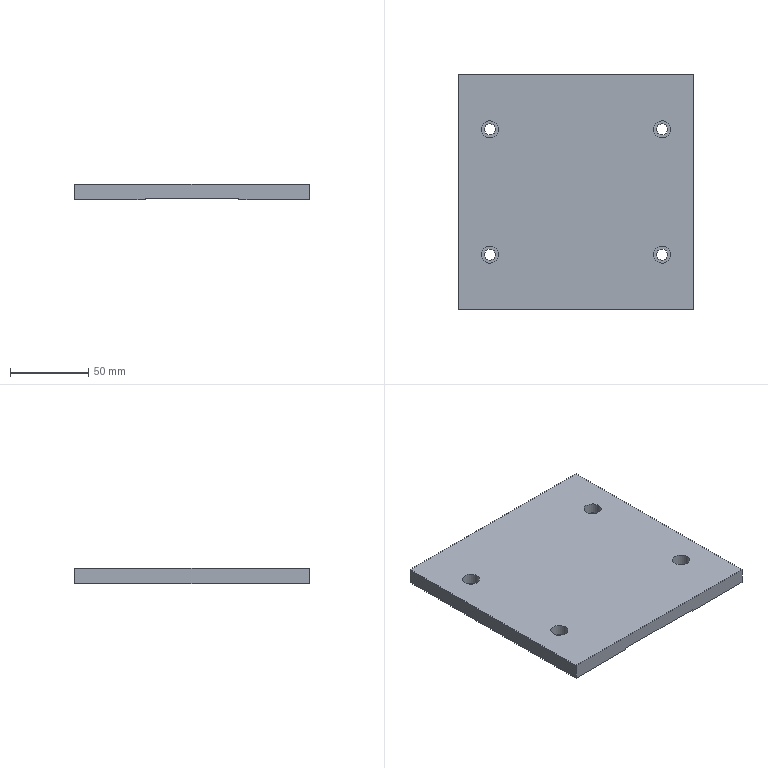Part | NX | features DATUM_CSYS 4, EXTRACT_BODY 3, EXTRUDE 3, SKETCH 3, Container 2, Geometry Instance 2, SUBTRACT 1 | 1 solid | 22 faces | box 150 x 150 x 10 mm | volume 212877 mm3 | plane 14 | cylinder 8 | commonest cylinder face diameters 7 x4 11 x4
STEP:
#1=CARTESIAN_POINT('',(0.,0.,10.));
#2=VERTEX_POINT('',#1);
#3=CARTESIAN_POINT('',(0.,0.,0.));
#4=VERTEX_POINT('',#3);
#5=CARTESIAN_POINT('',(0.,0.,10.));
#6=DIRECTION('',(0.,0.,-1.));
#7=VECTOR('',#6,1000.);
#8=LINE('',#5,#7);
#9=EDGE_CURVE('',#2,#4,#8,.T.);
#10=ORIENTED_EDGE('',*,*,#9,.F.);
#11=CARTESIAN_POINT('',(0.,150.,10.));
#12=VERTEX_POINT('',#11);
#13=CARTESIAN_POINT('',(0.,150.,10.));
#14=DIRECTION('',(0.,-1.,0.));
#15=VECTOR('',#14,1000.);
#16=LINE('',#13,#15);
#17=EDGE_CURVE('',#12,#2,#16,.T.);
#18=ORIENTED_EDGE('',*,*,#17,.F.);
#19=CARTESIAN_POINT('',(0.,150.,0.));
#20=VERTEX_POINT('',#19);
#21=CARTESIAN_POINT('',(0.,150.,10.));
#22=DIRECTION('',(0.,0.,-1.));
#23=VECTOR('',#22,1000.);
#24=LINE('',#21,#23);
#25=EDGE_CURVE('',#12,#20,#24,.T.);
#26=ORIENTED_EDGE('',*,*,#25,.T.);
#27=CARTESIAN_POINT('',(0.,150.,0.));
#28=DIRECTION('',(0.,-1.,0.));
#29=VECTOR('',#28,1000.);
#30=LINE('',#27,#29);
#31=EDGE_CURVE('',#20,#4,#30,.T.);
#32=ORIENTED_EDGE('',*,*,#31,.T.);
#33=EDGE_LOOP('',(#10,#18,#26,#32));
#34=FACE_BOUND('',#33,.T.);
#35=CARTESIAN_POINT('',(0.,150.,10.));
#36=DIRECTION('',(-1.,0.,0.));
#37=DIRECTION('',(0.,0.,1.));
#38=AXIS2_PLACEMENT_3D('',#35,#36,#37);
#39=PLANE('',#38);
#40=ADVANCED_FACE('',(#34),#39,.T.);
#41=CARTESIAN_POINT('',(16.5,35.,0.));
#42=VERTEX_POINT('',#41);
#43=CARTESIAN_POINT('',(20.,35.,0.));
#44=DIRECTION('',(0.,0.,1.));
#45=DIRECTION('',(-1.,0.,0.));
#46=AXIS2_PLACEMENT_3D('',#43,#44,#45);
#47=CIRCLE('',#46,3.5);
#48=EDGE_CURVE('',#42,#42,#47,.T.);
#49=ORIENTED_EDGE('',*,*,#48,.T.);
#50=EDGE_LOOP('',(#49));
#51=FACE_BOUND('',#50,.T.);
#52=CARTESIAN_POINT('',(16.5,115.,0.));
#53=VERTEX_POINT('',#52);
#54=CARTESIAN_POINT('',(20.,115.,0.));
#55=DIRECTION('',(0.,0.,-1.));
#56=DIRECTION('',(-1.,0.,0.));
#57=AXIS2_PLACEMENT_3D('',#54,#55,#56);
#58=CIRCLE('',#57,3.5);
#59=EDGE_CURVE('',#53,#53,#58,.F.);
#60=ORIENTED_EDGE('',*,*,#59,.T.);
#61=EDGE_LOOP('',(#60));
#62=FACE_BOUND('',#61,.T.);
#63=CARTESIAN_POINT('',(45.,0.,0.));
#64=VERTEX_POINT('',#63);
#65=CARTESIAN_POINT('',(0.,0.,0.));
#66=DIRECTION('',(1.,0.,0.));
#67=VECTOR('',#66,1000.);
#68=LINE('',#65,#67);
#69=EDGE_CURVE('',#4,#64,#68,.T.);
#70=ORIENTED_EDGE('',*,*,#69,.F.);
#71=ORIENTED_EDGE('',*,*,#31,.F.);
#72=CARTESIAN_POINT('',(45.,150.,0.));
#73=VERTEX_POINT('',#72);
#74=CARTESIAN_POINT('',(0.,150.,0.));
#75=DIRECTION('',(1.,0.,0.));
#76=VECTOR('',#75,1000.);
#77=LINE('',#74,#76);
#78=EDGE_CURVE('',#20,#73,#77,.T.);
#79=ORIENTED_EDGE('',*,*,#78,.T.);
#80=CARTESIAN_POINT('',(45.,150.,0.));
#81=DIRECTION('',(0.,-1.,0.));
#82=VECTOR('',#81,1000.);
#83=LINE('',#80,#82);
#84=EDGE_CURVE('',#73,#64,#83,.T.);
#85=ORIENTED_EDGE('',*,*,#84,.T.);
#86=EDGE_LOOP('',(#70,#71,#79,#85));
#87=FACE_BOUND('',#86,.T.);
#88=CARTESIAN_POINT('',(0.,150.,0.));
#89=DIRECTION('',(0.,0.,-1.));
#90=DIRECTION('',(-1.,0.,0.));
#91=AXIS2_PLACEMENT_3D('',#88,#89,#90);
#92=PLANE('',#91);
#93=ADVANCED_FACE('',(#51,#62,#87),#92,.T.);
#94=CARTESIAN_POINT('',(45.,0.,1.));
#95=VERTEX_POINT('',#94);
#96=CARTESIAN_POINT('',(45.,0.,0.));
#97=DIRECTION('',(0.,0.,1.));
#98=VECTOR('',#97,1000.);
#99=LINE('',#96,#98);
#100=EDGE_CURVE('',#64,#95,#99,.T.);
#101=ORIENTED_EDGE('',*,*,#100,.F.);
#102=ORIENTED_EDGE('',*,*,#84,.F.);
#103=CARTESIAN_POINT('',(45.,150.,1.));
#104=VERTEX_POINT('',#103);
#105=CARTESIAN_POINT('',(45.,150.,0.));
#106=DIRECTION('',(0.,0.,1.));
#107=VECTOR('',#106,1000.);
#108=LINE('',#105,#107);
#109=EDGE_CURVE('',#73,#104,#108,.T.);
#110=ORIENTED_EDGE('',*,*,#109,.T.);
#111=CARTESIAN_POINT('',(45.,150.,1.));
#112=DIRECTION('',(0.,-1.,0.));
#113=VECTOR('',#112,1000.);
#114=LINE('',#111,#113);
#115=EDGE_CURVE('',#104,#95,#114,.T.);
#116=ORIENTED_EDGE('',*,*,#115,.T.);
#117=EDGE_LOOP('',(#101,#102,#110,#116));
#118=FACE_BOUND('',#117,.T.);
#119=CARTESIAN_POINT('',(45.,150.,0.));
#120=DIRECTION('',(1.,0.,0.));
#121=DIRECTION('',(0.,0.,-1.));
#122=AXIS2_PLACEMENT_3D('',#119,#120,#121);
#123=PLANE('',#122);
#124=ADVANCED_FACE('',(#118),#123,.T.);
#125=CARTESIAN_POINT('',(105.,0.,1.));
#126=VERTEX_POINT('',#125);
#127=CARTESIAN_POINT('',(75.,0.,1.));
#128=DIRECTION('',(1.,0.,0.));
#129=VECTOR('',#128,1000.);
#130=LINE('',#127,#129);
#131=EDGE_CURVE('',#95,#126,#130,.T.);
#132=ORIENTED_EDGE('',*,*,#131,.F.);
#133=ORIENTED_EDGE('',*,*,#115,.F.);
#134=CARTESIAN_POINT('',(105.,150.,1.));
#135=VERTEX_POINT('',#134);
#136=CARTESIAN_POINT('',(45.,150.,1.));
#137=DIRECTION('',(1.,0.,0.));
#138=VECTOR('',#137,1000.);
#139=LINE('',#136,#138);
#140=EDGE_CURVE('',#104,#135,#139,.T.);
#141=ORIENTED_EDGE('',*,*,#140,.T.);
#142=CARTESIAN_POINT('',(105.,150.,1.));
#143=DIRECTION('',(0.,-1.,0.));
#144=VECTOR('',#143,1000.);
#145=LINE('',#142,#144);
#146=EDGE_CURVE('',#135,#126,#145,.T.);
#147=ORIENTED_EDGE('',*,*,#146,.T.);
#148=EDGE_LOOP('',(#132,#133,#141,#147));
#149=FACE_BOUND('',#148,.T.);
#150=CARTESIAN_POINT('',(75.,150.,1.));
#151=DIRECTION('',(0.,0.,-1.));
#152=DIRECTION('',(-1.,0.,0.));
#153=AXIS2_PLACEMENT_3D('',#150,#151,#152);
#154=PLANE('',#153);
#155=ADVANCED_FACE('',(#149),#154,.T.);
#156=CARTESIAN_POINT('',(105.,0.,0.));
#157=VERTEX_POINT('',#156);
#158=CARTESIAN_POINT('',(105.,0.,1.));
#159=DIRECTION('',(0.,0.,-1.));
#160=VECTOR('',#159,1000.);
#161=LINE('',#158,#160);
#162=EDGE_CURVE('',#126,#157,#161,.T.);
#163=ORIENTED_EDGE('',*,*,#162,.F.);
#164=ORIENTED_EDGE('',*,*,#146,.F.);
#165=CARTESIAN_POINT('',(105.,150.,0.));
#166=VERTEX_POINT('',#165);
#167=CARTESIAN_POINT('',(105.,150.,1.));
#168=DIRECTION('',(0.,0.,-1.));
#169=VECTOR('',#168,1000.);
#170=LINE('',#167,#169);
#171=EDGE_CURVE('',#135,#166,#170,.T.);
#172=ORIENTED_EDGE('',*,*,#171,.T.);
#173=CARTESIAN_POINT('',(105.,150.,0.));
#174=DIRECTION('',(0.,-1.,0.));
#175=VECTOR('',#174,1000.);
#176=LINE('',#173,#175);
#177=EDGE_CURVE('',#166,#157,#176,.T.);
#178=ORIENTED_EDGE('',*,*,#177,.T.);
#179=EDGE_LOOP('',(#163,#164,#172,#178));
#180=FACE_BOUND('',#179,.T.);
#181=CARTESIAN_POINT('',(105.,150.,1.));
#182=DIRECTION('',(-1.,0.,0.));
#183=DIRECTION('',(0.,0.,1.));
#184=AXIS2_PLACEMENT_3D('',#181,#182,#183);
#185=PLANE('',#184);
#186=ADVANCED_FACE('',(#180),#185,.T.);
#187=CARTESIAN_POINT('',(133.5,35.,0.));
#188=VERTEX_POINT('',#187);
#189=CARTESIAN_POINT('',(130.,35.,0.));
#190=DIRECTION('',(0.,0.,-1.));
#191=DIRECTION('',(1.,0.,0.));
#192=AXIS2_PLACEMENT_3D('',#189,#190,#191);
#193=CIRCLE('',#192,3.5);
#194=EDGE_CURVE('',#188,#188,#193,.F.);
#195=ORIENTED_EDGE('',*,*,#194,.T.);
#196=EDGE_LOOP('',(#195));
#197=FACE_BOUND('',#196,.T.);
#198=CARTESIAN_POINT('',(133.5,115.,0.));
#199=VERTEX_POINT('',#198);
#200=CARTESIAN_POINT('',(130.,115.,0.));
#201=DIRECTION('',(0.,0.,1.));
#202=DIRECTION('',(1.,0.,0.));
#203=AXIS2_PLACEMENT_3D('',#200,#201,#202);
#204=CIRCLE('',#203,3.5);
#205=EDGE_CURVE('',#199,#199,#204,.T.);
#206=ORIENTED_EDGE('',*,*,#205,.T.);
#207=EDGE_LOOP('',(#206));
#208=FACE_BOUND('',#207,.T.);
#209=CARTESIAN_POINT('',(150.,0.,0.));
#210=VERTEX_POINT('',#209);
#211=CARTESIAN_POINT('',(105.,0.,0.));
#212=DIRECTION('',(1.,0.,0.));
#213=VECTOR('',#212,1000.);
#214=LINE('',#211,#213);
#215=EDGE_CURVE('',#157,#210,#214,.T.);
#216=ORIENTED_EDGE('',*,*,#215,.F.);
#217=ORIENTED_EDGE('',*,*,#177,.F.);
#218=CARTESIAN_POINT('',(150.,150.,0.));
#219=VERTEX_POINT('',#218);
#220=CARTESIAN_POINT('',(105.,150.,0.));
#221=DIRECTION('',(1.,0.,0.));
#222=VECTOR('',#221,1000.);
#223=LINE('',#220,#222);
#224=EDGE_CURVE('',#166,#219,#223,.T.);
#225=ORIENTED_EDGE('',*,*,#224,.T.);
#226=CARTESIAN_POINT('',(150.,150.,0.));
#227=DIRECTION('',(0.,-1.,0.));
#228=VECTOR('',#227,1000.);
#229=LINE('',#226,#228);
#230=EDGE_CURVE('',#219,#210,#229,.T.);
#231=ORIENTED_EDGE('',*,*,#230,.T.);
#232=EDGE_LOOP('',(#216,#217,#225,#231));
#233=FACE_BOUND('',#232,.T.);
#234=CARTESIAN_POINT('',(105.,150.,0.));
#235=DIRECTION('',(0.,0.,-1.));
#236=DIRECTION('',(-1.,0.,0.));
#237=AXIS2_PLACEMENT_3D('',#234,#235,#236);
#238=PLANE('',#237);
#239=ADVANCED_FACE('',(#197,#208,#233),#238,.T.);
#240=CARTESIAN_POINT('',(150.,0.,10.));
#241=VERTEX_POINT('',#240);
#242=CARTESIAN_POINT('',(150.,0.,0.));
#243=DIRECTION('',(0.,0.,1.));
#244=VECTOR('',#243,1000.);
#245=LINE('',#242,#244);
#246=EDGE_CURVE('',#210,#241,#245,.T.);
#247=ORIENTED_EDGE('',*,*,#246,.F.);
#248=ORIENTED_EDGE('',*,*,#230,.F.);
#249=CARTESIAN_POINT('',(150.,150.,10.));
#250=VERTEX_POINT('',#249);
#251=CARTESIAN_POINT('',(150.,150.,0.));
#252=DIRECTION('',(0.,0.,1.));
#253=VECTOR('',#252,1000.);
#254=LINE('',#251,#253);
#255=EDGE_CURVE('',#219,#250,#254,.T.);
#256=ORIENTED_EDGE('',*,*,#255,.T.);
#257=CARTESIAN_POINT('',(150.,150.,10.));
#258=DIRECTION('',(0.,-1.,0.));
#259=VECTOR('',#258,1000.);
#260=LINE('',#257,#259);
#261=EDGE_CURVE('',#250,#241,#260,.T.);
#262=ORIENTED_EDGE('',*,*,#261,.T.);
#263=EDGE_LOOP('',(#247,#248,#256,#262));
#264=FACE_BOUND('',#263,.T.);
#265=CARTESIAN_POINT('',(150.,150.,0.));
#266=DIRECTION('',(1.,0.,0.));
#267=DIRECTION('',(0.,0.,-1.));
#268=AXIS2_PLACEMENT_3D('',#265,#266,#267);
#269=PLANE('',#268);
#270=ADVANCED_FACE('',(#264),#269,.T.);
#271=CARTESIAN_POINT('',(135.5,35.,10.));
#272=VERTEX_POINT('',#271);
#273=CARTESIAN_POINT('',(130.,35.,10.));
#274=DIRECTION('',(0.,0.,-1.));
#275=DIRECTION('',(1.,0.,0.));
#276=AXIS2_PLACEMENT_3D('',#273,#274,#275);
#277=CIRCLE('',#276,5.5);
#278=EDGE_CURVE('',#272,#272,#277,.F.);
#279=ORIENTED_EDGE('',*,*,#278,.F.);
#280=EDGE_LOOP('',(#279));
#281=FACE_BOUND('',#280,.T.);
#282=CARTESIAN_POINT('',(14.5,35.,10.));
#283=VERTEX_POINT('',#282);
#284=CARTESIAN_POINT('',(20.,35.,10.));
#285=DIRECTION('',(0.,0.,1.));
#286=DIRECTION('',(-1.,0.,0.));
#287=AXIS2_PLACEMENT_3D('',#284,#285,#286);
#288=CIRCLE('',#287,5.5);
#289=EDGE_CURVE('',#283,#283,#288,.T.);
#290=ORIENTED_EDGE('',*,*,#289,.F.);
#291=EDGE_LOOP('',(#290));
#292=FACE_BOUND('',#291,.T.);
#293=CARTESIAN_POINT('',(14.5,115.,10.));
#294=VERTEX_POINT('',#293);
#295=CARTESIAN_POINT('',(20.,115.,10.));
#296=DIRECTION('',(0.,0.,-1.));
#297=DIRECTION('',(-1.,0.,0.));
#298=AXIS2_PLACEMENT_3D('',#295,#296,#297);
#299=CIRCLE('',#298,5.5);
#300=EDGE_CURVE('',#294,#294,#299,.F.);
#301=ORIENTED_EDGE('',*,*,#300,.F.);
#302=EDGE_LOOP('',(#301));
#303=FACE_BOUND('',#302,.T.);
#304=CARTESIAN_POINT('',(135.5,115.,10.));
#305=VERTEX_POINT('',#304);
#306=CARTESIAN_POINT('',(130.,115.,10.));
#307=DIRECTION('',(0.,0.,1.));
#308=DIRECTION('',(1.,0.,0.));
#309=AXIS2_PLACEMENT_3D('',#306,#307,#308);
#310=CIRCLE('',#309,5.5);
#311=EDGE_CURVE('',#305,#305,#310,.T.);
#312=ORIENTED_EDGE('',*,*,#311,.F.);
#313=EDGE_LOOP('',(#312));
#314=FACE_BOUND('',#313,.T.);
#315=CARTESIAN_POINT('',(150.,0.,10.));
#316=DIRECTION('',(-1.,0.,0.));
#317=VECTOR('',#316,1000.);
#318=LINE('',#315,#317);
#319=EDGE_CURVE('',#241,#2,#318,.T.);
#320=ORIENTED_EDGE('',*,*,#319,.F.);
#321=ORIENTED_EDGE('',*,*,#261,.F.);
#322=CARTESIAN_POINT('',(150.,150.,10.));
#323=DIRECTION('',(-1.,0.,0.));
#324=VECTOR('',#323,1000.);
#325=LINE('',#322,#324);
#326=EDGE_CURVE('',#250,#12,#325,.T.);
#327=ORIENTED_EDGE('',*,*,#326,.T.);
#328=ORIENTED_EDGE('',*,*,#17,.T.);
#329=EDGE_LOOP('',(#320,#321,#327,#328));
#330=FACE_BOUND('',#329,.T.);
#331=CARTESIAN_POINT('',(150.,150.,10.));
#332=DIRECTION('',(0.,0.,1.));
#333=DIRECTION('',(1.,0.,0.));
#334=AXIS2_PLACEMENT_3D('',#331,#332,#333);
#335=PLANE('',#334);
#336=ADVANCED_FACE('',(#281,#292,#303,#314,#330),#335,.T.);
#337=ORIENTED_EDGE('',*,*,#25,.F.);
#338=ORIENTED_EDGE('',*,*,#326,.F.);
#339=ORIENTED_EDGE('',*,*,#255,.F.);
#340=ORIENTED_EDGE('',*,*,#224,.F.);
#341=ORIENTED_EDGE('',*,*,#171,.F.);
#342=ORIENTED_EDGE('',*,*,#140,.F.);
#343=ORIENTED_EDGE('',*,*,#109,.F.);
#344=ORIENTED_EDGE('',*,*,#78,.F.);
#345=EDGE_LOOP('',(#337,#338,#339,#340,#341,#342,#343,#344));
#346=FACE_BOUND('',#345,.T.);
#347=CARTESIAN_POINT('',(0.,150.,0.));
#348=DIRECTION('',(0.,-1.,0.));
#349=DIRECTION('',(0.,0.,-1.));
#350=AXIS2_PLACEMENT_3D('',#347,#348,#349);
#351=PLANE('',#350);
#352=ADVANCED_FACE('',(#346),#351,.F.);
#353=ORIENTED_EDGE('',*,*,#9,.T.);
#354=ORIENTED_EDGE('',*,*,#69,.T.);
#355=ORIENTED_EDGE('',*,*,#100,.T.);
#356=ORIENTED_EDGE('',*,*,#131,.T.);
#357=ORIENTED_EDGE('',*,*,#162,.T.);
#358=ORIENTED_EDGE('',*,*,#215,.T.);
#359=ORIENTED_EDGE('',*,*,#246,.T.);
#360=ORIENTED_EDGE('',*,*,#319,.T.);
#361=EDGE_LOOP('',(#353,#354,#355,#356,#357,#358,#359,#360));
#362=FACE_BOUND('',#361,.T.);
#363=CARTESIAN_POINT('',(0.,0.,0.));
#364=DIRECTION('',(0.,-1.,0.));
#365=DIRECTION('',(0.,0.,-1.));
#366=AXIS2_PLACEMENT_3D('',#363,#364,#365);
#367=PLANE('',#366);
#368=ADVANCED_FACE('',(#362),#367,.T.);
#369=CARTESIAN_POINT('',(135.5,115.,3.));
#370=VERTEX_POINT('',#369);
#371=CARTESIAN_POINT('',(130.,115.,3.));
#372=DIRECTION('',(0.,0.,1.));
#373=DIRECTION('',(1.,0.,0.));
#374=AXIS2_PLACEMENT_3D('',#371,#372,#373);
#375=CIRCLE('',#374,5.5);
#376=EDGE_CURVE('',#370,#370,#375,.F.);
#377=ORIENTED_EDGE('',*,*,#376,.T.);
#378=EDGE_LOOP('',(#377));
#379=FACE_BOUND('',#378,.T.);
#380=ORIENTED_EDGE('',*,*,#311,.T.);
#381=EDGE_LOOP('',(#380));
#382=FACE_BOUND('',#381,.T.);
#383=CARTESIAN_POINT('',(130.,115.,3.));
#384=DIRECTION('',(0.,0.,1.));
#385=DIRECTION('',(1.,0.,0.));
#386=AXIS2_PLACEMENT_3D('',#383,#384,#385);
#387=CYLINDRICAL_SURFACE('',#386,5.5);
#388=ADVANCED_FACE('',(#379,#382),#387,.F.);
#389=CARTESIAN_POINT('',(133.5,115.,3.));
#390=VERTEX_POINT('',#389);
#391=CARTESIAN_POINT('',(130.,115.,3.));
#392=DIRECTION('',(0.,0.,1.));
#393=DIRECTION('',(1.,0.,0.));
#394=AXIS2_PLACEMENT_3D('',#391,#392,#393);
#395=CIRCLE('',#394,3.5);
#396=EDGE_CURVE('',#390,#390,#395,.F.);
#397=ORIENTED_EDGE('',*,*,#396,.T.);
#398=EDGE_LOOP('',(#397));
#399=FACE_BOUND('',#398,.T.);
#400=ORIENTED_EDGE('',*,*,#376,.F.);
#401=EDGE_LOOP('',(#400));
#402=FACE_BOUND('',#401,.T.);
#403=CARTESIAN_POINT('',(130.,115.,3.));
#404=DIRECTION('',(0.,0.,1.));
#405=DIRECTION('',(1.,0.,0.));
#406=AXIS2_PLACEMENT_3D('',#403,#404,#405);
#407=PLANE('',#406);
#408=ADVANCED_FACE('',(#399,#402),#407,.T.);
#409=ORIENTED_EDGE('',*,*,#205,.F.);
#410=EDGE_LOOP('',(#409));
#411=FACE_BOUND('',#410,.T.);
#412=ORIENTED_EDGE('',*,*,#396,.F.);
#413=EDGE_LOOP('',(#412));
#414=FACE_BOUND('',#413,.T.);
#415=CARTESIAN_POINT('',(130.,115.,0.));
#416=DIRECTION('',(0.,0.,1.));
#417=DIRECTION('',(1.,0.,0.));
#418=AXIS2_PLACEMENT_3D('',#415,#416,#417);
#419=CYLINDRICAL_SURFACE('',#418,3.5);
#420=ADVANCED_FACE('',(#411,#414),#419,.F.);
#421=CARTESIAN_POINT('',(14.5,115.,3.));
#422=VERTEX_POINT('',#421);
#423=CARTESIAN_POINT('',(20.,115.,3.));
#424=DIRECTION('',(0.,0.,-1.));
#425=DIRECTION('',(-1.,0.,0.));
#426=AXIS2_PLACEMENT_3D('',#423,#424,#425);
#427=CIRCLE('',#426,5.5);
#428=EDGE_CURVE('',#422,#422,#427,.T.);
#429=ORIENTED_EDGE('',*,*,#428,.T.);
#430=EDGE_LOOP('',(#429));
#431=FACE_BOUND('',#430,.T.);
#432=ORIENTED_EDGE('',*,*,#300,.T.);
#433=EDGE_LOOP('',(#432));
#434=FACE_BOUND('',#433,.T.);
#435=CARTESIAN_POINT('',(20.,115.,3.));
#436=DIRECTION('',(0.,0.,1.));
#437=DIRECTION('',(-1.,0.,0.));
#438=AXIS2_PLACEMENT_3D('',#435,#436,#437);
#439=CYLINDRICAL_SURFACE('',#438,5.5);
#440=ADVANCED_FACE('',(#431,#434),#439,.F.);
#441=CARTESIAN_POINT('',(16.5,115.,3.));
#442=VERTEX_POINT('',#441);
#443=CARTESIAN_POINT('',(20.,115.,3.));
#444=DIRECTION('',(0.,0.,-1.));
#445=DIRECTION('',(-1.,0.,0.));
#446=AXIS2_PLACEMENT_3D('',#443,#444,#445);
#447=CIRCLE('',#446,3.5);
#448=EDGE_CURVE('',#442,#442,#447,.T.);
#449=ORIENTED_EDGE('',*,*,#448,.T.);
#450=EDGE_LOOP('',(#449));
#451=FACE_BOUND('',#450,.T.);
#452=ORIENTED_EDGE('',*,*,#428,.F.);
#453=EDGE_LOOP('',(#452));
#454=FACE_BOUND('',#453,.T.);
#455=CARTESIAN_POINT('',(20.,115.,3.));
#456=DIRECTION('',(0.,0.,1.));
#457=DIRECTION('',(-1.,0.,0.));
#458=AXIS2_PLACEMENT_3D('',#455,#456,#457);
#459=PLANE('',#458);
#460=ADVANCED_FACE('',(#451,#454),#459,.T.);
#461=ORIENTED_EDGE('',*,*,#59,.F.);
#462=EDGE_LOOP('',(#461));
#463=FACE_BOUND('',#462,.T.);
#464=ORIENTED_EDGE('',*,*,#448,.F.);
#465=EDGE_LOOP('',(#464));
#466=FACE_BOUND('',#465,.T.);
#467=CARTESIAN_POINT('',(20.,115.,0.));
#468=DIRECTION('',(0.,0.,1.));
#469=DIRECTION('',(-1.,0.,0.));
#470=AXIS2_PLACEMENT_3D('',#467,#468,#469);
#471=CYLINDRICAL_SURFACE('',#470,3.5);
#472=ADVANCED_FACE('',(#463,#466),#471,.F.);
#473=CARTESIAN_POINT('',(14.5,35.,3.));
#474=VERTEX_POINT('',#473);
#475=CARTESIAN_POINT('',(20.,35.,3.));
#476=DIRECTION('',(0.,0.,1.));
#477=DIRECTION('',(-1.,0.,0.));
#478=AXIS2_PLACEMENT_3D('',#475,#476,#477);
#479=CIRCLE('',#478,5.5);
#480=EDGE_CURVE('',#474,#474,#479,.F.);
#481=ORIENTED_EDGE('',*,*,#480,.T.);
#482=EDGE_LOOP('',(#481));
#483=FACE_BOUND('',#482,.T.);
#484=ORIENTED_EDGE('',*,*,#289,.T.);
#485=EDGE_LOOP('',(#484));
#486=FACE_BOUND('',#485,.T.);
#487=CARTESIAN_POINT('',(20.,35.,3.));
#488=DIRECTION('',(0.,0.,1.));
#489=DIRECTION('',(-1.,0.,0.));
#490=AXIS2_PLACEMENT_3D('',#487,#488,#489);
#491=CYLINDRICAL_SURFACE('',#490,5.5);
#492=ADVANCED_FACE('',(#483,#486),#491,.F.);
#493=CARTESIAN_POINT('',(16.5,35.,3.));
#494=VERTEX_POINT('',#493);
#495=CARTESIAN_POINT('',(20.,35.,3.));
#496=DIRECTION('',(0.,0.,1.));
#497=DIRECTION('',(-1.,0.,0.));
#498=AXIS2_PLACEMENT_3D('',#495,#496,#497);
#499=CIRCLE('',#498,3.5);
#500=EDGE_CURVE('',#494,#494,#499,.F.);
#501=ORIENTED_EDGE('',*,*,#500,.T.);
#502=EDGE_LOOP('',(#501));
#503=FACE_BOUND('',#502,.T.);
#504=ORIENTED_EDGE('',*,*,#480,.F.);
#505=EDGE_LOOP('',(#504));
#506=FACE_BOUND('',#505,.T.);
#507=CARTESIAN_POINT('',(20.,35.,3.));
#508=DIRECTION('',(0.,0.,1.));
#509=DIRECTION('',(-1.,0.,0.));
#510=AXIS2_PLACEMENT_3D('',#507,#508,#509);
#511=PLANE('',#510);
#512=ADVANCED_FACE('',(#503,#506),#511,.T.);
#513=ORIENTED_EDGE('',*,*,#48,.F.);
#514=EDGE_LOOP('',(#513));
#515=FACE_BOUND('',#514,.T.);
#516=ORIENTED_EDGE('',*,*,#500,.F.);
#517=EDGE_LOOP('',(#516));
#518=FACE_BOUND('',#517,.T.);
#519=CARTESIAN_POINT('',(20.,35.,0.));
#520=DIRECTION('',(0.,0.,1.));
#521=DIRECTION('',(-1.,0.,0.));
#522=AXIS2_PLACEMENT_3D('',#519,#520,#521);
#523=CYLINDRICAL_SURFACE('',#522,3.5);
#524=ADVANCED_FACE('',(#515,#518),#523,.F.);
#525=CARTESIAN_POINT('',(135.5,35.,3.));
#526=VERTEX_POINT('',#525);
#527=CARTESIAN_POINT('',(130.,35.,3.));
#528=DIRECTION('',(0.,0.,-1.));
#529=DIRECTION('',(1.,0.,0.));
#530=AXIS2_PLACEMENT_3D('',#527,#528,#529);
#531=CIRCLE('',#530,5.5);
#532=EDGE_CURVE('',#526,#526,#531,.T.);
#533=ORIENTED_EDGE('',*,*,#532,.T.);
#534=EDGE_LOOP('',(#533));
#535=FACE_BOUND('',#534,.T.);
#536=ORIENTED_EDGE('',*,*,#278,.T.);
#537=EDGE_LOOP('',(#536));
#538=FACE_BOUND('',#537,.T.);
#539=CARTESIAN_POINT('',(130.,35.,3.));
#540=DIRECTION('',(0.,0.,1.));
#541=DIRECTION('',(1.,0.,0.));
#542=AXIS2_PLACEMENT_3D('',#539,#540,#541);
#543=CYLINDRICAL_SURFACE('',#542,5.5);
#544=ADVANCED_FACE('',(#535,#538),#543,.F.);
#545=CARTESIAN_POINT('',(133.5,35.,3.));
#546=VERTEX_POINT('',#545);
#547=CARTESIAN_POINT('',(130.,35.,3.));
#548=DIRECTION('',(0.,0.,-1.));
#549=DIRECTION('',(1.,0.,0.));
#550=AXIS2_PLACEMENT_3D('',#547,#548,#549);
#551=CIRCLE('',#550,3.5);
#552=EDGE_CURVE('',#546,#546,#551,.T.);
#553=ORIENTED_EDGE('',*,*,#552,.T.);
#554=EDGE_LOOP('',(#553));
#555=FACE_BOUND('',#554,.T.);
#556=ORIENTED_EDGE('',*,*,#532,.F.);
#557=EDGE_LOOP('',(#556));
#558=FACE_BOUND('',#557,.T.);
#559=CARTESIAN_POINT('',(130.,35.,3.));
#560=DIRECTION('',(0.,0.,1.));
#561=DIRECTION('',(1.,0.,0.));
#562=AXIS2_PLACEMENT_3D('',#559,#560,#561);
#563=PLANE('',#562);
#564=ADVANCED_FACE('',(#555,#558),#563,.T.);
#565=ORIENTED_EDGE('',*,*,#194,.F.);
#566=EDGE_LOOP('',(#565));
#567=FACE_BOUND('',#566,.T.);
#568=ORIENTED_EDGE('',*,*,#552,.F.);
#569=EDGE_LOOP('',(#568));
#570=FACE_BOUND('',#569,.T.);
#571=CARTESIAN_POINT('',(130.,35.,0.));
#572=DIRECTION('',(0.,0.,1.));
#573=DIRECTION('',(1.,0.,0.));
#574=AXIS2_PLACEMENT_3D('',#571,#572,#573);
#575=CYLINDRICAL_SURFACE('',#574,3.5);
#576=ADVANCED_FACE('',(#567,#570),#575,.F.);
#577=CLOSED_SHELL('',(#40,#93,#124,#155,#186,#239,#270,#336,#352,#368,#388,#408,#420,#440,#460,#472,#492,#512,#524,#544,#564,#576));
#578=MANIFOLD_SOLID_BREP('',#577);
#579=(LENGTH_UNIT()NAMED_UNIT(*)SI_UNIT(.MILLI.,.METRE.));
#580=UNCERTAINTY_MEASURE_WITH_UNIT(LENGTH_MEASURE(0.00001),#579,'','');
#581=(NAMED_UNIT(*)PLANE_ANGLE_UNIT()SI_UNIT($,.RADIAN.));
#582=(NAMED_UNIT(*)SI_UNIT($,.STERADIAN.)SOLID_ANGLE_UNIT());
#583=(GEOMETRIC_REPRESENTATION_CONTEXT(3)GLOBAL_UNCERTAINTY_ASSIGNED_CONTEXT((#580))GLOBAL_UNIT_ASSIGNED_CONTEXT((#579,#581,#582))REPRESENTATION_CONTEXT('',''));
#584=ADVANCED_BREP_SHAPE_REPRESENTATION('',(#578),#583);